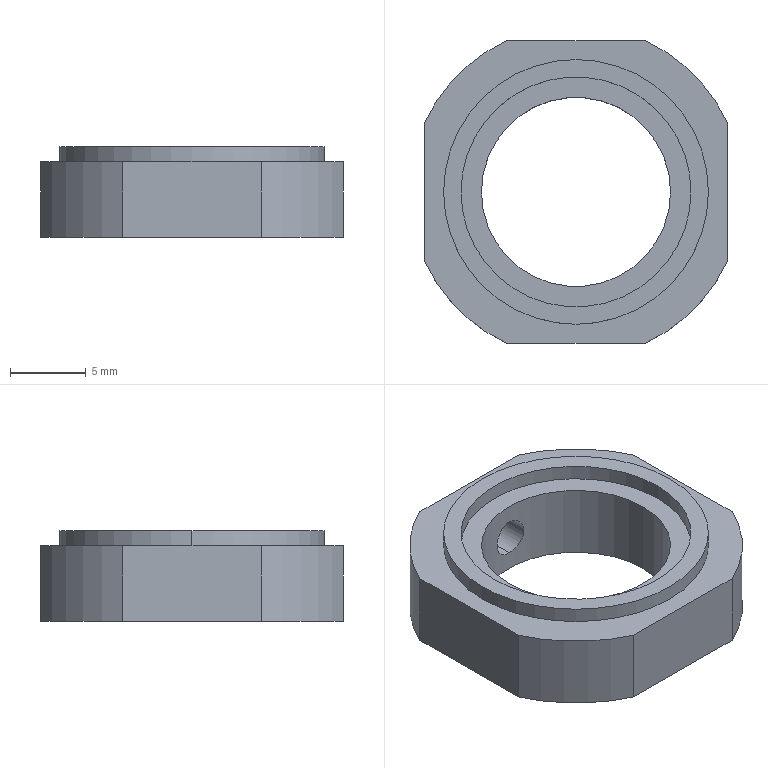Part | SolidWorks | features HoleWzd 2, ICE 2, Extrusion 1 | 1 solid | 20 faces | box 20 x 20 x 6 mm | volume 1204 mm3 | cylinder 12 | plane 8 | commonest cylinder face diameters 22 x4 2.5 x2 12.5 x2 15.2 x2 17.5 x2
STEP:
#1=CARTESIAN_POINT('',(0.,6.25,-1.25));
#2=VERTEX_POINT('',#1);
#3=CARTESIAN_POINT('',(0.,6.25,1.25));
#4=VERTEX_POINT('',#3);
#5=CARTESIAN_POINT('',(0.,6.25,-1.25));
#6=CARTESIAN_POINT('',(-0.1633,6.25,-1.25));
#7=CARTESIAN_POINT('',(-0.3282,6.243,-1.217));
#8=CARTESIAN_POINT('',(-0.6292,6.22,-1.092));
#9=CARTESIAN_POINT('',(-0.7681,6.204,-0.9995));
#10=CARTESIAN_POINT('',(-0.9987,6.171,-0.7692));
#11=CARTESIAN_POINT('',(-1.091,6.154,-0.6315));
#12=CARTESIAN_POINT('',(-1.217,6.131,-0.3282));
#13=CARTESIAN_POINT('',(-1.25,6.124,-0.1657));
#14=CARTESIAN_POINT('',(-1.25,6.124,0.1644));
#15=CARTESIAN_POINT('',(-1.217,6.131,0.3276));
#16=CARTESIAN_POINT('',(-1.092,6.154,0.6296));
#17=CARTESIAN_POINT('',(-0.9993,6.171,0.7684));
#18=CARTESIAN_POINT('',(-0.7696,6.204,0.9983));
#19=CARTESIAN_POINT('',(-0.6306,6.22,1.091));
#20=CARTESIAN_POINT('',(-0.33,6.243,1.217));
#21=CARTESIAN_POINT('',(-0.1656,6.25,1.25));
#22=CARTESIAN_POINT('',(0.,6.25,1.25));
#23=B_SPLINE_CURVE_WITH_KNOTS('',3,(#5,#6,#7,#8,#9,#10,#11,#12,#13,#14,#15,#16,#17,#18,#19,#20,#21,#22),.UNSPECIFIED.,.F.,.F.,(4,2,2,2,2,2,2,2,4),(0.003918,0.004408,0.004897,0.005387,0.005876,0.006366,0.006856,0.007345,0.007835),.UNSPECIFIED.);
#24=EDGE_CURVE('',#2,#4,#23,.T.);
#25=ORIENTED_EDGE('',*,*,#24,.F.);
#26=CARTESIAN_POINT('',(0.,10.,-1.25));
#27=VERTEX_POINT('',#26);
#28=CARTESIAN_POINT('',(0.,10.,-1.25));
#29=DIRECTION('',(0.,1.,0.));
#30=VECTOR('',#29,1000.);
#31=LINE('',#28,#30);
#32=EDGE_CURVE('',#2,#27,#31,.T.);
#33=ORIENTED_EDGE('',*,*,#32,.T.);
#34=CARTESIAN_POINT('',(0.,10.,1.25));
#35=VERTEX_POINT('',#34);
#36=CARTESIAN_POINT('',(0.,10.,0.));
#37=DIRECTION('',(0.,1.,0.));
#38=DIRECTION('',(0.,0.,1.));
#39=AXIS2_PLACEMENT_3D('',#36,#37,#38);
#40=CIRCLE('',#39,1.25);
#41=EDGE_CURVE('',#27,#35,#40,.T.);
#42=ORIENTED_EDGE('',*,*,#41,.T.);
#43=CARTESIAN_POINT('',(0.,10.,1.25));
#44=DIRECTION('',(0.,1.,0.));
#45=VECTOR('',#44,1000.);
#46=LINE('',#43,#45);
#47=EDGE_CURVE('',#4,#35,#46,.T.);
#48=ORIENTED_EDGE('',*,*,#47,.F.);
#49=EDGE_LOOP('',(#25,#33,#42,#48));
#50=FACE_OUTER_BOUND('',#49,.T.);
#51=CARTESIAN_POINT('',(0.,10.,0.));
#52=DIRECTION('',(0.,1.,0.));
#53=DIRECTION('',(0.,0.,1.));
#54=AXIS2_PLACEMENT_3D('',#51,#52,#53);
#55=CYLINDRICAL_SURFACE('',#54,1.25);
#56=ADVANCED_FACE('',(#50),#55,.F.);
#57=CARTESIAN_POINT('',(-6.25,0.,2.5));
#58=VERTEX_POINT('',#57);
#59=CARTESIAN_POINT('',(6.25,0.,2.5));
#60=VERTEX_POINT('',#59);
#61=CARTESIAN_POINT('',(0.,0.,2.5));
#62=DIRECTION('',(0.,0.,1.));
#63=DIRECTION('',(1.,0.,0.));
#64=AXIS2_PLACEMENT_3D('',#61,#62,#63);
#65=CIRCLE('',#64,6.25);
#66=EDGE_CURVE('',#58,#60,#65,.T.);
#67=ORIENTED_EDGE('',*,*,#66,.T.);
#68=CARTESIAN_POINT('',(6.25,0.,-2.5));
#69=VERTEX_POINT('',#68);
#70=CARTESIAN_POINT('',(6.25,0.,-2.5));
#71=DIRECTION('',(0.,0.,-1.));
#72=VECTOR('',#71,1000.);
#73=LINE('',#70,#72);
#74=EDGE_CURVE('',#60,#69,#73,.T.);
#75=ORIENTED_EDGE('',*,*,#74,.T.);
#76=CARTESIAN_POINT('',(-6.25,0.,-2.5));
#77=VERTEX_POINT('',#76);
#78=CARTESIAN_POINT('',(0.,0.,-2.5));
#79=DIRECTION('',(0.,0.,-1.));
#80=DIRECTION('',(-1.,0.,0.));
#81=AXIS2_PLACEMENT_3D('',#78,#79,#80);
#82=CIRCLE('',#81,6.25);
#83=EDGE_CURVE('',#69,#77,#82,.T.);
#84=ORIENTED_EDGE('',*,*,#83,.T.);
#85=CARTESIAN_POINT('',(-6.25,0.,-2.5));
#86=DIRECTION('',(0.,0.,-1.));
#87=VECTOR('',#86,1000.);
#88=LINE('',#85,#87);
#89=EDGE_CURVE('',#58,#77,#88,.T.);
#90=ORIENTED_EDGE('',*,*,#89,.F.);
#91=EDGE_LOOP('',(#67,#75,#84,#90));
#92=FACE_OUTER_BOUND('',#91,.T.);
#93=CARTESIAN_POINT('',(0.,0.,-2.5));
#94=DIRECTION('',(0.,0.,-1.));
#95=DIRECTION('',(-1.,0.,0.));
#96=AXIS2_PLACEMENT_3D('',#93,#94,#95);
#97=CYLINDRICAL_SURFACE('',#96,6.25);
#98=ADVANCED_FACE('',(#92),#97,.F.);
#99=CARTESIAN_POINT('',(-7.6,0.,3.5));
#100=VERTEX_POINT('',#99);
#101=CARTESIAN_POINT('',(7.6,0.,3.5));
#102=VERTEX_POINT('',#101);
#103=CARTESIAN_POINT('',(0.,0.,3.5));
#104=DIRECTION('',(0.,0.,1.));
#105=DIRECTION('',(1.,0.,0.));
#106=AXIS2_PLACEMENT_3D('',#103,#104,#105);
#107=CIRCLE('',#106,7.6);
#108=EDGE_CURVE('',#100,#102,#107,.T.);
#109=ORIENTED_EDGE('',*,*,#108,.T.);
#110=CARTESIAN_POINT('',(7.6,0.,2.5));
#111=VERTEX_POINT('',#110);
#112=CARTESIAN_POINT('',(7.6,0.,3.5));
#113=DIRECTION('',(0.,0.,-1.));
#114=VECTOR('',#113,1000.);
#115=LINE('',#112,#114);
#116=EDGE_CURVE('',#102,#111,#115,.T.);
#117=ORIENTED_EDGE('',*,*,#116,.T.);
#118=CARTESIAN_POINT('',(-7.6,0.,2.5));
#119=VERTEX_POINT('',#118);
#120=CARTESIAN_POINT('',(0.,0.,2.5));
#121=DIRECTION('',(0.,0.,-1.));
#122=DIRECTION('',(1.,0.,0.));
#123=AXIS2_PLACEMENT_3D('',#120,#121,#122);
#124=CIRCLE('',#123,7.6);
#125=EDGE_CURVE('',#111,#119,#124,.T.);
#126=ORIENTED_EDGE('',*,*,#125,.T.);
#127=CARTESIAN_POINT('',(-7.6,0.,3.5));
#128=DIRECTION('',(0.,0.,-1.));
#129=VECTOR('',#128,1000.);
#130=LINE('',#127,#129);
#131=EDGE_CURVE('',#100,#119,#130,.T.);
#132=ORIENTED_EDGE('',*,*,#131,.F.);
#133=EDGE_LOOP('',(#109,#117,#126,#132));
#134=FACE_OUTER_BOUND('',#133,.T.);
#135=CARTESIAN_POINT('',(0.,0.,3.5));
#136=DIRECTION('',(0.,0.,-1.));
#137=DIRECTION('',(-1.,0.,0.));
#138=AXIS2_PLACEMENT_3D('',#135,#136,#137);
#139=CYLINDRICAL_SURFACE('',#138,7.6);
#140=ADVANCED_FACE('',(#134),#139,.F.);
#141=CARTESIAN_POINT('',(8.75,0.,3.5));
#142=VERTEX_POINT('',#141);
#143=CARTESIAN_POINT('',(-8.75,0.,3.5));
#144=VERTEX_POINT('',#143);
#145=CARTESIAN_POINT('',(0.,0.,3.5));
#146=DIRECTION('',(0.,0.,1.));
#147=DIRECTION('',(1.,0.,0.));
#148=AXIS2_PLACEMENT_3D('',#145,#146,#147);
#149=CIRCLE('',#148,8.75);
#150=EDGE_CURVE('',#142,#144,#149,.T.);
#151=ORIENTED_EDGE('',*,*,#150,.F.);
#152=CARTESIAN_POINT('',(8.75,0.,2.5));
#153=VERTEX_POINT('',#152);
#154=CARTESIAN_POINT('',(8.75,0.,3.5));
#155=DIRECTION('',(0.,0.,-1.));
#156=VECTOR('',#155,1000.);
#157=LINE('',#154,#156);
#158=EDGE_CURVE('',#142,#153,#157,.T.);
#159=ORIENTED_EDGE('',*,*,#158,.T.);
#160=CARTESIAN_POINT('',(-8.75,0.,2.5));
#161=VERTEX_POINT('',#160);
#162=CARTESIAN_POINT('',(0.,0.,2.5));
#163=DIRECTION('',(0.,0.,1.));
#164=DIRECTION('',(1.,0.,0.));
#165=AXIS2_PLACEMENT_3D('',#162,#163,#164);
#166=CIRCLE('',#165,8.75);
#167=EDGE_CURVE('',#153,#161,#166,.T.);
#168=ORIENTED_EDGE('',*,*,#167,.T.);
#169=CARTESIAN_POINT('',(-8.75,0.,3.5));
#170=DIRECTION('',(0.,0.,-1.));
#171=VECTOR('',#170,1000.);
#172=LINE('',#169,#171);
#173=EDGE_CURVE('',#144,#161,#172,.T.);
#174=ORIENTED_EDGE('',*,*,#173,.F.);
#175=EDGE_LOOP('',(#151,#159,#168,#174));
#176=FACE_OUTER_BOUND('',#175,.T.);
#177=CARTESIAN_POINT('',(0.,0.,3.5));
#178=DIRECTION('',(0.,0.,-1.));
#179=DIRECTION('',(-1.,0.,0.));
#180=AXIS2_PLACEMENT_3D('',#177,#178,#179);
#181=CYLINDRICAL_SURFACE('',#180,8.75);
#182=ADVANCED_FACE('',(#176),#181,.T.);
#183=CARTESIAN_POINT('',(0.,0.,2.5));
#184=DIRECTION('',(0.,0.,1.));
#185=DIRECTION('',(1.,0.,0.));
#186=AXIS2_PLACEMENT_3D('',#183,#184,#185);
#187=CIRCLE('',#186,8.75);
#188=EDGE_CURVE('',#161,#153,#187,.T.);
#189=ORIENTED_EDGE('',*,*,#188,.F.);
#190=ORIENTED_EDGE('',*,*,#167,.F.);
#191=EDGE_LOOP('',(#189,#190));
#192=FACE_BOUND('',#191,.T.);
#193=CARTESIAN_POINT('',(-4.583,10.,2.5));
#194=VERTEX_POINT('',#193);
#195=CARTESIAN_POINT('',(-10.,4.583,2.5));
#196=VERTEX_POINT('',#195);
#197=CARTESIAN_POINT('',(0.,0.,2.5));
#198=DIRECTION('',(0.,0.,1.));
#199=DIRECTION('',(1.,0.,0.));
#200=AXIS2_PLACEMENT_3D('',#197,#198,#199);
#201=CIRCLE('',#200,11.);
#202=EDGE_CURVE('',#194,#196,#201,.T.);
#203=ORIENTED_EDGE('',*,*,#202,.T.);
#204=CARTESIAN_POINT('',(-10.,-4.583,2.5));
#205=VERTEX_POINT('',#204);
#206=CARTESIAN_POINT('',(-10.,0.,2.5));
#207=DIRECTION('',(0.,-1.,0.));
#208=VECTOR('',#207,1000.);
#209=LINE('',#206,#208);
#210=EDGE_CURVE('',#196,#205,#209,.T.);
#211=ORIENTED_EDGE('',*,*,#210,.T.);
#212=CARTESIAN_POINT('',(-4.583,-10.,2.5));
#213=VERTEX_POINT('',#212);
#214=CARTESIAN_POINT('',(0.,0.,2.5));
#215=DIRECTION('',(0.,0.,1.));
#216=DIRECTION('',(1.,0.,0.));
#217=AXIS2_PLACEMENT_3D('',#214,#215,#216);
#218=CIRCLE('',#217,11.);
#219=EDGE_CURVE('',#205,#213,#218,.T.);
#220=ORIENTED_EDGE('',*,*,#219,.T.);
#221=CARTESIAN_POINT('',(4.583,-10.,2.5));
#222=VERTEX_POINT('',#221);
#223=CARTESIAN_POINT('',(0.,-10.,2.5));
#224=DIRECTION('',(1.,0.,0.));
#225=VECTOR('',#224,1000.);
#226=LINE('',#223,#225);
#227=EDGE_CURVE('',#213,#222,#226,.T.);
#228=ORIENTED_EDGE('',*,*,#227,.T.);
#229=CARTESIAN_POINT('',(10.,-4.583,2.5));
#230=VERTEX_POINT('',#229);
#231=CARTESIAN_POINT('',(0.,0.,2.5));
#232=DIRECTION('',(0.,0.,1.));
#233=DIRECTION('',(1.,0.,0.));
#234=AXIS2_PLACEMENT_3D('',#231,#232,#233);
#235=CIRCLE('',#234,11.);
#236=EDGE_CURVE('',#222,#230,#235,.T.);
#237=ORIENTED_EDGE('',*,*,#236,.T.);
#238=CARTESIAN_POINT('',(10.,4.583,2.5));
#239=VERTEX_POINT('',#238);
#240=CARTESIAN_POINT('',(10.,0.,2.5));
#241=DIRECTION('',(0.,1.,0.));
#242=VECTOR('',#241,1000.);
#243=LINE('',#240,#242);
#244=EDGE_CURVE('',#230,#239,#243,.T.);
#245=ORIENTED_EDGE('',*,*,#244,.T.);
#246=CARTESIAN_POINT('',(4.583,10.,2.5));
#247=VERTEX_POINT('',#246);
#248=CARTESIAN_POINT('',(0.,0.,2.5));
#249=DIRECTION('',(0.,0.,1.));
#250=DIRECTION('',(1.,0.,0.));
#251=AXIS2_PLACEMENT_3D('',#248,#249,#250);
#252=CIRCLE('',#251,11.);
#253=EDGE_CURVE('',#239,#247,#252,.T.);
#254=ORIENTED_EDGE('',*,*,#253,.T.);
#255=CARTESIAN_POINT('',(0.,10.,2.5));
#256=DIRECTION('',(-1.,0.,0.));
#257=VECTOR('',#256,1000.);
#258=LINE('',#255,#257);
#259=EDGE_CURVE('',#247,#194,#258,.T.);
#260=ORIENTED_EDGE('',*,*,#259,.T.);
#261=EDGE_LOOP('',(#203,#211,#220,#228,#237,#245,#254,#260));
#262=FACE_OUTER_BOUND('',#261,.T.);
#263=CARTESIAN_POINT('',(0.,0.,2.5));
#264=DIRECTION('',(0.,0.,1.));
#265=DIRECTION('',(1.,0.,0.));
#266=AXIS2_PLACEMENT_3D('',#263,#264,#265);
#267=PLANE('',#266);
#268=ADVANCED_FACE('',(#192,#262),#267,.T.);
#269=CARTESIAN_POINT('',(-10.,4.583,-2.5));
#270=VERTEX_POINT('',#269);
#271=CARTESIAN_POINT('',(-10.,4.583,2.5));
#272=DIRECTION('',(0.,0.,-1.));
#273=VECTOR('',#272,1000.);
#274=LINE('',#271,#273);
#275=EDGE_CURVE('',#196,#270,#274,.T.);
#276=ORIENTED_EDGE('',*,*,#275,.F.);
#277=ORIENTED_EDGE('',*,*,#202,.F.);
#278=CARTESIAN_POINT('',(-4.583,10.,-2.5));
#279=VERTEX_POINT('',#278);
#280=CARTESIAN_POINT('',(-4.583,10.,2.5));
#281=DIRECTION('',(0.,0.,1.));
#282=VECTOR('',#281,1000.);
#283=LINE('',#280,#282);
#284=EDGE_CURVE('',#279,#194,#283,.T.);
#285=ORIENTED_EDGE('',*,*,#284,.F.);
#286=CARTESIAN_POINT('',(0.,0.,-2.5));
#287=DIRECTION('',(0.,0.,1.));
#288=DIRECTION('',(1.,0.,0.));
#289=AXIS2_PLACEMENT_3D('',#286,#287,#288);
#290=CIRCLE('',#289,11.);
#291=EDGE_CURVE('',#279,#270,#290,.T.);
#292=ORIENTED_EDGE('',*,*,#291,.T.);
#293=EDGE_LOOP('',(#276,#277,#285,#292));
#294=FACE_OUTER_BOUND('',#293,.T.);
#295=CARTESIAN_POINT('',(0.,0.,2.5));
#296=DIRECTION('',(0.,0.,-1.));
#297=DIRECTION('',(-1.,0.,0.));
#298=AXIS2_PLACEMENT_3D('',#295,#296,#297);
#299=CYLINDRICAL_SURFACE('',#298,11.);
#300=ADVANCED_FACE('',(#294),#299,.T.);
#301=CARTESIAN_POINT('',(-10.,-4.583,-2.5));
#302=VERTEX_POINT('',#301);
#303=CARTESIAN_POINT('',(-10.,-4.583,2.5));
#304=DIRECTION('',(0.,0.,1.));
#305=VECTOR('',#304,1000.);
#306=LINE('',#303,#305);
#307=EDGE_CURVE('',#302,#205,#306,.T.);
#308=ORIENTED_EDGE('',*,*,#307,.F.);
#309=CARTESIAN_POINT('',(-4.583,-10.,-2.5));
#310=VERTEX_POINT('',#309);
#311=CARTESIAN_POINT('',(0.,0.,-2.5));
#312=DIRECTION('',(0.,0.,1.));
#313=DIRECTION('',(1.,0.,0.));
#314=AXIS2_PLACEMENT_3D('',#311,#312,#313);
#315=CIRCLE('',#314,11.);
#316=EDGE_CURVE('',#302,#310,#315,.T.);
#317=ORIENTED_EDGE('',*,*,#316,.T.);
#318=CARTESIAN_POINT('',(-4.583,-10.,2.5));
#319=DIRECTION('',(0.,0.,-1.));
#320=VECTOR('',#319,1000.);
#321=LINE('',#318,#320);
#322=EDGE_CURVE('',#213,#310,#321,.T.);
#323=ORIENTED_EDGE('',*,*,#322,.F.);
#324=ORIENTED_EDGE('',*,*,#219,.F.);
#325=EDGE_LOOP('',(#308,#317,#323,#324));
#326=FACE_OUTER_BOUND('',#325,.T.);
#327=CARTESIAN_POINT('',(0.,0.,2.5));
#328=DIRECTION('',(0.,0.,-1.));
#329=DIRECTION('',(-1.,0.,0.));
#330=AXIS2_PLACEMENT_3D('',#327,#328,#329);
#331=CYLINDRICAL_SURFACE('',#330,11.);
#332=ADVANCED_FACE('',(#326),#331,.T.);
#333=CARTESIAN_POINT('',(4.583,-10.,-2.5));
#334=VERTEX_POINT('',#333);
#335=CARTESIAN_POINT('',(4.583,-10.,2.5));
#336=DIRECTION('',(0.,0.,1.));
#337=VECTOR('',#336,1000.);
#338=LINE('',#335,#337);
#339=EDGE_CURVE('',#334,#222,#338,.T.);
#340=ORIENTED_EDGE('',*,*,#339,.F.);
#341=CARTESIAN_POINT('',(10.,-4.583,-2.5));
#342=VERTEX_POINT('',#341);
#343=CARTESIAN_POINT('',(0.,0.,-2.5));
#344=DIRECTION('',(0.,0.,1.));
#345=DIRECTION('',(1.,0.,0.));
#346=AXIS2_PLACEMENT_3D('',#343,#344,#345);
#347=CIRCLE('',#346,11.);
#348=EDGE_CURVE('',#334,#342,#347,.T.);
#349=ORIENTED_EDGE('',*,*,#348,.T.);
#350=CARTESIAN_POINT('',(10.,-4.583,2.5));
#351=DIRECTION('',(0.,0.,-1.));
#352=VECTOR('',#351,1000.);
#353=LINE('',#350,#352);
#354=EDGE_CURVE('',#230,#342,#353,.T.);
#355=ORIENTED_EDGE('',*,*,#354,.F.);
#356=ORIENTED_EDGE('',*,*,#236,.F.);
#357=EDGE_LOOP('',(#340,#349,#355,#356));
#358=FACE_OUTER_BOUND('',#357,.T.);
#359=CARTESIAN_POINT('',(0.,0.,2.5));
#360=DIRECTION('',(0.,0.,-1.));
#361=DIRECTION('',(-1.,0.,0.));
#362=AXIS2_PLACEMENT_3D('',#359,#360,#361);
#363=CYLINDRICAL_SURFACE('',#362,11.);
#364=ADVANCED_FACE('',(#358),#363,.T.);
#365=CARTESIAN_POINT('',(10.,4.583,-2.5));
#366=VERTEX_POINT('',#365);
#367=CARTESIAN_POINT('',(10.,4.583,2.5));
#368=DIRECTION('',(0.,0.,1.));
#369=VECTOR('',#368,1000.);
#370=LINE('',#367,#369);
#371=EDGE_CURVE('',#366,#239,#370,.T.);
#372=ORIENTED_EDGE('',*,*,#371,.F.);
#373=CARTESIAN_POINT('',(4.583,10.,-2.5));
#374=VERTEX_POINT('',#373);
#375=CARTESIAN_POINT('',(0.,0.,-2.5));
#376=DIRECTION('',(0.,0.,1.));
#377=DIRECTION('',(1.,0.,0.));
#378=AXIS2_PLACEMENT_3D('',#375,#376,#377);
#379=CIRCLE('',#378,11.);
#380=EDGE_CURVE('',#366,#374,#379,.T.);
#381=ORIENTED_EDGE('',*,*,#380,.T.);
#382=CARTESIAN_POINT('',(4.583,10.,2.5));
#383=DIRECTION('',(0.,0.,-1.));
#384=VECTOR('',#383,1000.);
#385=LINE('',#382,#384);
#386=EDGE_CURVE('',#247,#374,#385,.T.);
#387=ORIENTED_EDGE('',*,*,#386,.F.);
#388=ORIENTED_EDGE('',*,*,#253,.F.);
#389=EDGE_LOOP('',(#372,#381,#387,#388));
#390=FACE_OUTER_BOUND('',#389,.T.);
#391=CARTESIAN_POINT('',(0.,0.,2.5));
#392=DIRECTION('',(0.,0.,-1.));
#393=DIRECTION('',(-1.,0.,0.));
#394=AXIS2_PLACEMENT_3D('',#391,#392,#393);
#395=CYLINDRICAL_SURFACE('',#394,11.);
#396=ADVANCED_FACE('',(#390),#395,.T.);
#397=CARTESIAN_POINT('',(0.,0.,-2.5));
#398=DIRECTION('',(0.,0.,-1.));
#399=DIRECTION('',(-1.,0.,0.));
#400=AXIS2_PLACEMENT_3D('',#397,#398,#399);
#401=CIRCLE('',#400,6.25);
#402=EDGE_CURVE('',#77,#69,#401,.T.);
#403=ORIENTED_EDGE('',*,*,#402,.F.);
#404=ORIENTED_EDGE('',*,*,#83,.F.);
#405=EDGE_LOOP('',(#403,#404));
#406=FACE_BOUND('',#405,.T.);
#407=CARTESIAN_POINT('',(-10.,0.,-2.5));
#408=DIRECTION('',(0.,-1.,0.));
#409=VECTOR('',#408,1000.);
#410=LINE('',#407,#409);
#411=EDGE_CURVE('',#270,#302,#410,.T.);
#412=ORIENTED_EDGE('',*,*,#411,.F.);
#413=ORIENTED_EDGE('',*,*,#291,.F.);
#414=CARTESIAN_POINT('',(0.,10.,-2.5));
#415=DIRECTION('',(-1.,0.,0.));
#416=VECTOR('',#415,1000.);
#417=LINE('',#414,#416);
#418=EDGE_CURVE('',#374,#279,#417,.T.);
#419=ORIENTED_EDGE('',*,*,#418,.F.);
#420=ORIENTED_EDGE('',*,*,#380,.F.);
#421=CARTESIAN_POINT('',(10.,0.,-2.5));
#422=DIRECTION('',(0.,1.,0.));
#423=VECTOR('',#422,1000.);
#424=LINE('',#421,#423);
#425=EDGE_CURVE('',#342,#366,#424,.T.);
#426=ORIENTED_EDGE('',*,*,#425,.F.);
#427=ORIENTED_EDGE('',*,*,#348,.F.);
#428=CARTESIAN_POINT('',(0.,-10.,-2.5));
#429=DIRECTION('',(1.,0.,0.));
#430=VECTOR('',#429,1000.);
#431=LINE('',#428,#430);
#432=EDGE_CURVE('',#310,#334,#431,.T.);
#433=ORIENTED_EDGE('',*,*,#432,.F.);
#434=ORIENTED_EDGE('',*,*,#316,.F.);
#435=EDGE_LOOP('',(#412,#413,#419,#420,#426,#427,#433,#434));
#436=FACE_OUTER_BOUND('',#435,.T.);
#437=CARTESIAN_POINT('',(0.,0.,-2.5));
#438=DIRECTION('',(0.,0.,1.));
#439=DIRECTION('',(1.,0.,0.));
#440=AXIS2_PLACEMENT_3D('',#437,#438,#439);
#441=PLANE('',#440);
#442=ADVANCED_FACE('',(#406,#436),#441,.F.);
#443=CARTESIAN_POINT('',(0.,0.,3.5));
#444=DIRECTION('',(0.,0.,1.));
#445=DIRECTION('',(1.,0.,0.));
#446=AXIS2_PLACEMENT_3D('',#443,#444,#445);
#447=CIRCLE('',#446,8.75);
#448=EDGE_CURVE('',#144,#142,#447,.T.);
#449=ORIENTED_EDGE('',*,*,#448,.T.);
#450=ORIENTED_EDGE('',*,*,#150,.T.);
#451=EDGE_LOOP('',(#449,#450));
#452=FACE_OUTER_BOUND('',#451,.T.);
#453=ORIENTED_EDGE('',*,*,#108,.F.);
#454=CARTESIAN_POINT('',(0.,0.,3.5));
#455=DIRECTION('',(0.,0.,1.));
#456=DIRECTION('',(1.,0.,0.));
#457=AXIS2_PLACEMENT_3D('',#454,#455,#456);
#458=CIRCLE('',#457,7.6);
#459=EDGE_CURVE('',#102,#100,#458,.T.);
#460=ORIENTED_EDGE('',*,*,#459,.F.);
#461=EDGE_LOOP('',(#453,#460));
#462=FACE_BOUND('',#461,.T.);
#463=CARTESIAN_POINT('',(0.,0.,3.5));
#464=DIRECTION('',(0.,0.,1.));
#465=DIRECTION('',(1.,0.,0.));
#466=AXIS2_PLACEMENT_3D('',#463,#464,#465);
#467=PLANE('',#466);
#468=ADVANCED_FACE('',(#452,#462),#467,.T.);
#469=ORIENTED_EDGE('',*,*,#158,.F.);
#470=ORIENTED_EDGE('',*,*,#448,.F.);
#471=ORIENTED_EDGE('',*,*,#173,.T.);
#472=ORIENTED_EDGE('',*,*,#188,.T.);
#473=EDGE_LOOP('',(#469,#470,#471,#472));
#474=FACE_OUTER_BOUND('',#473,.T.);
#475=CARTESIAN_POINT('',(0.,0.,3.5));
#476=DIRECTION('',(0.,0.,-1.));
#477=DIRECTION('',(-1.,0.,0.));
#478=AXIS2_PLACEMENT_3D('',#475,#476,#477);
#479=CYLINDRICAL_SURFACE('',#478,8.75);
#480=ADVANCED_FACE('',(#474),#479,.T.);
#481=ORIENTED_EDGE('',*,*,#116,.F.);
#482=ORIENTED_EDGE('',*,*,#459,.T.);
#483=ORIENTED_EDGE('',*,*,#131,.T.);
#484=CARTESIAN_POINT('',(0.,0.,2.5));
#485=DIRECTION('',(0.,0.,-1.));
#486=DIRECTION('',(1.,0.,0.));
#487=AXIS2_PLACEMENT_3D('',#484,#485,#486);
#488=CIRCLE('',#487,7.6);
#489=EDGE_CURVE('',#119,#111,#488,.T.);
#490=ORIENTED_EDGE('',*,*,#489,.T.);
#491=EDGE_LOOP('',(#481,#482,#483,#490));
#492=FACE_OUTER_BOUND('',#491,.T.);
#493=CARTESIAN_POINT('',(0.,0.,3.5));
#494=DIRECTION('',(0.,0.,-1.));
#495=DIRECTION('',(-1.,0.,0.));
#496=AXIS2_PLACEMENT_3D('',#493,#494,#495);
#497=CYLINDRICAL_SURFACE('',#496,7.6);
#498=ADVANCED_FACE('',(#492),#497,.F.);
#499=ORIENTED_EDGE('',*,*,#66,.F.);
#500=CARTESIAN_POINT('',(0.,0.,2.5));
#501=DIRECTION('',(0.,0.,1.));
#502=DIRECTION('',(1.,0.,0.));
#503=AXIS2_PLACEMENT_3D('',#500,#501,#502);
#504=CIRCLE('',#503,6.25);
#505=EDGE_CURVE('',#60,#58,#504,.T.);
#506=ORIENTED_EDGE('',*,*,#505,.F.);
#507=EDGE_LOOP('',(#499,#506));
#508=FACE_BOUND('',#507,.T.);
#509=ORIENTED_EDGE('',*,*,#489,.F.);
#510=ORIENTED_EDGE('',*,*,#125,.F.);
#511=EDGE_LOOP('',(#509,#510));
#512=FACE_OUTER_BOUND('',#511,.T.);
#513=CARTESIAN_POINT('',(0.,0.,2.5));
#514=DIRECTION('',(0.,0.,1.));
#515=DIRECTION('',(1.,0.,0.));
#516=AXIS2_PLACEMENT_3D('',#513,#514,#515);
#517=PLANE('',#516);
#518=ADVANCED_FACE('',(#508,#512),#517,.T.);
#519=ORIENTED_EDGE('',*,*,#74,.F.);
#520=ORIENTED_EDGE('',*,*,#505,.T.);
#521=ORIENTED_EDGE('',*,*,#89,.T.);
#522=ORIENTED_EDGE('',*,*,#402,.T.);
#523=EDGE_LOOP('',(#519,#520,#521,#522));
#524=FACE_OUTER_BOUND('',#523,.T.);
#525=CARTESIAN_POINT('',(0.,6.25,1.25));
#526=CARTESIAN_POINT('',(0.1656,6.25,1.25));
#527=CARTESIAN_POINT('',(0.3281,6.243,1.217));
#528=CARTESIAN_POINT('',(0.6307,6.22,1.092));
#529=CARTESIAN_POINT('',(0.7691,6.204,0.9987));
#530=CARTESIAN_POINT('',(0.9991,6.171,0.7686));
#531=CARTESIAN_POINT('',(1.092,6.154,0.6295));
#532=CARTESIAN_POINT('',(1.217,6.131,0.3288));
#533=CARTESIAN_POINT('',(1.25,6.124,0.164));
#534=CARTESIAN_POINT('',(1.25,6.124,-0.08127));
#535=CARTESIAN_POINT('',(1.242,6.125,-0.1643));
#536=CARTESIAN_POINT('',(1.21,6.132,-0.3248));
#537=CARTESIAN_POINT('',(1.186,6.136,-0.4029));
#538=CARTESIAN_POINT('',(1.092,6.154,-0.6303));
#539=CARTESIAN_POINT('',(1.,6.171,-0.7678));
#540=CARTESIAN_POINT('',(0.7676,6.204,-1.));
#541=CARTESIAN_POINT('',(0.6299,6.22,-1.092));
#542=CARTESIAN_POINT('',(0.3277,6.243,-1.217));
#543=CARTESIAN_POINT('',(0.1634,6.25,-1.25));
#544=CARTESIAN_POINT('',(0.,6.25,-1.25));
#545=B_SPLINE_CURVE_WITH_KNOTS('',3,(#525,#526,#527,#528,#529,#530,#531,#532,#533,#534,#535,#536,#537,#538,#539,#540,#541,#542,#543,#544),.UNSPECIFIED.,.F.,.F.,(4,2,2,2,2,2,2,2,2,4),(0.,0.0004897,0.0009795,0.001469,0.001959,0.002204,0.002449,0.002938,0.003428,0.003918),.UNSPECIFIED.);
#546=EDGE_CURVE('',#4,#2,#545,.T.);
#547=ORIENTED_EDGE('',*,*,#546,.T.);
#548=ORIENTED_EDGE('',*,*,#24,.T.);
#549=EDGE_LOOP('',(#547,#548));
#550=FACE_BOUND('',#549,.T.);
#551=CARTESIAN_POINT('',(0.,0.,-2.5));
#552=DIRECTION('',(0.,0.,-1.));
#553=DIRECTION('',(-1.,0.,0.));
#554=AXIS2_PLACEMENT_3D('',#551,#552,#553);
#555=CYLINDRICAL_SURFACE('',#554,6.25);
#556=ADVANCED_FACE('',(#524,#550),#555,.F.);
#557=CARTESIAN_POINT('',(0.,10.,0.));
#558=DIRECTION('',(0.,1.,0.));
#559=DIRECTION('',(0.,0.,1.));
#560=AXIS2_PLACEMENT_3D('',#557,#558,#559);
#561=CIRCLE('',#560,1.25);
#562=EDGE_CURVE('',#35,#27,#561,.T.);
#563=ORIENTED_EDGE('',*,*,#562,.F.);
#564=ORIENTED_EDGE('',*,*,#41,.F.);
#565=EDGE_LOOP('',(#563,#564));
#566=FACE_BOUND('',#565,.T.);
#567=ORIENTED_EDGE('',*,*,#386,.T.);
#568=ORIENTED_EDGE('',*,*,#418,.T.);
#569=ORIENTED_EDGE('',*,*,#284,.T.);
#570=ORIENTED_EDGE('',*,*,#259,.F.);
#571=EDGE_LOOP('',(#567,#568,#569,#570));
#572=FACE_OUTER_BOUND('',#571,.T.);
#573=CARTESIAN_POINT('',(10.,10.,3.5));
#574=DIRECTION('',(0.,1.,0.));
#575=DIRECTION('',(0.,0.,1.));
#576=AXIS2_PLACEMENT_3D('',#573,#574,#575);
#577=PLANE('',#576);
#578=ADVANCED_FACE('',(#566,#572),#577,.T.);
#579=ORIENTED_EDGE('',*,*,#354,.T.);
#580=ORIENTED_EDGE('',*,*,#425,.T.);
#581=ORIENTED_EDGE('',*,*,#371,.T.);
#582=ORIENTED_EDGE('',*,*,#244,.F.);
#583=EDGE_LOOP('',(#579,#580,#581,#582));
#584=FACE_OUTER_BOUND('',#583,.T.);
#585=CARTESIAN_POINT('',(10.,10.,3.5));
#586=DIRECTION('',(1.,0.,0.));
#587=DIRECTION('',(0.,1.,0.));
#588=AXIS2_PLACEMENT_3D('',#585,#586,#587);
#589=PLANE('',#588);
#590=ADVANCED_FACE('',(#584),#589,.T.);
#591=ORIENTED_EDGE('',*,*,#322,.T.);
#592=ORIENTED_EDGE('',*,*,#432,.T.);
#593=ORIENTED_EDGE('',*,*,#339,.T.);
#594=ORIENTED_EDGE('',*,*,#227,.F.);
#595=EDGE_LOOP('',(#591,#592,#593,#594));
#596=FACE_OUTER_BOUND('',#595,.T.);
#597=CARTESIAN_POINT('',(10.,-10.,3.5));
#598=DIRECTION('',(0.,-1.,0.));
#599=DIRECTION('',(0.,0.,-1.));
#600=AXIS2_PLACEMENT_3D('',#597,#598,#599);
#601=PLANE('',#600);
#602=ADVANCED_FACE('',(#596),#601,.T.);
#603=ORIENTED_EDGE('',*,*,#275,.T.);
#604=ORIENTED_EDGE('',*,*,#411,.T.);
#605=ORIENTED_EDGE('',*,*,#307,.T.);
#606=ORIENTED_EDGE('',*,*,#210,.F.);
#607=EDGE_LOOP('',(#603,#604,#605,#606));
#608=FACE_OUTER_BOUND('',#607,.T.);
#609=CARTESIAN_POINT('',(-10.,10.,3.5));
#610=DIRECTION('',(-1.,0.,0.));
#611=DIRECTION('',(0.,-1.,0.));
#612=AXIS2_PLACEMENT_3D('',#609,#610,#611);
#613=PLANE('',#612);
#614=ADVANCED_FACE('',(#608),#613,.T.);
#615=ORIENTED_EDGE('',*,*,#32,.F.);
#616=ORIENTED_EDGE('',*,*,#546,.F.);
#617=ORIENTED_EDGE('',*,*,#47,.T.);
#618=ORIENTED_EDGE('',*,*,#562,.T.);
#619=EDGE_LOOP('',(#615,#616,#617,#618));
#620=FACE_OUTER_BOUND('',#619,.T.);
#621=CARTESIAN_POINT('',(0.,10.,0.));
#622=DIRECTION('',(0.,1.,0.));
#623=DIRECTION('',(0.,0.,1.));
#624=AXIS2_PLACEMENT_3D('',#621,#622,#623);
#625=CYLINDRICAL_SURFACE('',#624,1.25);
#626=ADVANCED_FACE('',(#620),#625,.F.);
#627=CLOSED_SHELL('',(#56,#98,#140,#182,#268,#300,#332,#364,#396,#442,#468,#480,#498,#518,#556,#578,#590,#602,#614,#626));
#628=MANIFOLD_SOLID_BREP('',#627);
#629=CARTESIAN_POINT('',(0.,0.,0.));
#630=DIRECTION('',(0.,0.,1.));
#631=DIRECTION('',(1.,0.,0.));
#632=AXIS2_PLACEMENT_3D('',#629,#630,#631);
#633=(LENGTH_UNIT()NAMED_UNIT(*)SI_UNIT(.MILLI.,.METRE.));
#634=UNCERTAINTY_MEASURE_WITH_UNIT(LENGTH_MEASURE(0.00001),#633,'','');
#635=(NAMED_UNIT(*)PLANE_ANGLE_UNIT()SI_UNIT($,.RADIAN.));
#636=(NAMED_UNIT(*)SI_UNIT($,.STERADIAN.)SOLID_ANGLE_UNIT());
#637=(GEOMETRIC_REPRESENTATION_CONTEXT(3)GLOBAL_UNCERTAINTY_ASSIGNED_CONTEXT((#634))GLOBAL_UNIT_ASSIGNED_CONTEXT((#633,#635,#636))REPRESENTATION_CONTEXT('',''));
#638=ADVANCED_BREP_SHAPE_REPRESENTATION('',(#628,#632),#637);